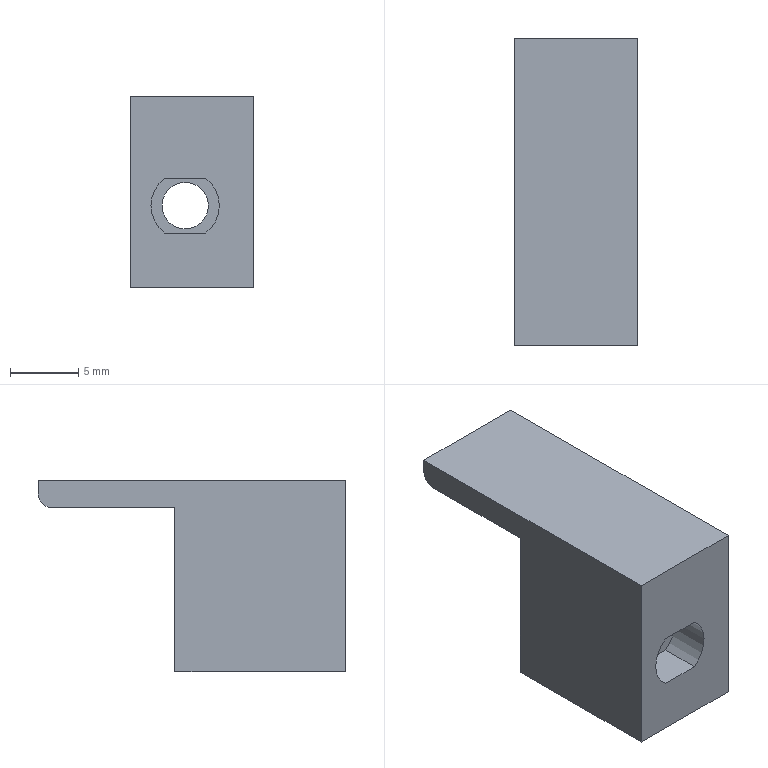Part | SolidWorks | features 3DProfileFeature 1, Cut 1, Extrusion 1, Fillet 1, HoleWzd 1, ICE 1 | 1 solid | 19 faces | box 9 x 22.5 x 14 mm | volume 1549 mm3 | plane 12 | cylinder 7 | commonest cylinder face diameters 3.4 x2 5 x2 6 x2 2 x1
STEP:
#1=CARTESIAN_POINT('',(-0.5,9.1,-4.));
#2=VERTEX_POINT('',#1);
#3=CARTESIAN_POINT('',(-0.5,9.1,2.));
#4=VERTEX_POINT('',#3);
#5=CARTESIAN_POINT('',(-0.5,9.1,-1.));
#6=DIRECTION('',(0.,1.,0.));
#7=DIRECTION('',(0.,0.,1.));
#8=AXIS2_PLACEMENT_3D('',#5,#6,#7);
#9=CIRCLE('',#8,3.);
#10=EDGE_CURVE('',#2,#4,#9,.T.);
#11=ORIENTED_EDGE('',*,*,#10,.F.);
#12=CARTESIAN_POINT('',(-0.5,12.5,-4.));
#13=VERTEX_POINT('',#12);
#14=CARTESIAN_POINT('',(-0.5,12.5,-4.));
#15=DIRECTION('',(0.,1.,0.));
#16=VECTOR('',#15,1000.);
#17=LINE('',#14,#16);
#18=EDGE_CURVE('',#2,#13,#17,.T.);
#19=ORIENTED_EDGE('',*,*,#18,.T.);
#20=CARTESIAN_POINT('',(-0.5,12.5,2.));
#21=VERTEX_POINT('',#20);
#22=CARTESIAN_POINT('',(-0.5,12.5,-1.));
#23=DIRECTION('',(0.,1.,0.));
#24=DIRECTION('',(0.,0.,1.));
#25=AXIS2_PLACEMENT_3D('',#22,#23,#24);
#26=CIRCLE('',#25,3.);
#27=EDGE_CURVE('',#13,#21,#26,.T.);
#28=ORIENTED_EDGE('',*,*,#27,.T.);
#29=CARTESIAN_POINT('',(-0.5,12.5,2.));
#30=DIRECTION('',(0.,1.,0.));
#31=VECTOR('',#30,1000.);
#32=LINE('',#29,#31);
#33=EDGE_CURVE('',#4,#21,#32,.T.);
#34=ORIENTED_EDGE('',*,*,#33,.F.);
#35=EDGE_LOOP('',(#11,#19,#28,#34));
#36=FACE_OUTER_BOUND('',#35,.T.);
#37=CARTESIAN_POINT('',(-0.5,12.5,-1.));
#38=DIRECTION('',(0.,1.,0.));
#39=DIRECTION('',(0.,0.,1.));
#40=AXIS2_PLACEMENT_3D('',#37,#38,#39);
#41=CYLINDRICAL_SURFACE('',#40,3.);
#42=ADVANCED_FACE('',(#36),#41,.F.);
#43=CARTESIAN_POINT('',(-0.5,3.,0.7));
#44=VERTEX_POINT('',#43);
#45=CARTESIAN_POINT('',(-0.5,3.,-2.7));
#46=VERTEX_POINT('',#45);
#47=CARTESIAN_POINT('',(-0.5,3.,-1.));
#48=DIRECTION('',(0.,-1.,0.));
#49=DIRECTION('',(0.,0.,-1.));
#50=AXIS2_PLACEMENT_3D('',#47,#48,#49);
#51=CIRCLE('',#50,1.7);
#52=EDGE_CURVE('',#44,#46,#51,.T.);
#53=ORIENTED_EDGE('',*,*,#52,.T.);
#54=CARTESIAN_POINT('',(-0.5,9.1,-2.7));
#55=VERTEX_POINT('',#54);
#56=CARTESIAN_POINT('',(-0.5,12.5,-2.7));
#57=DIRECTION('',(0.,1.,0.));
#58=VECTOR('',#57,1000.);
#59=LINE('',#56,#58);
#60=EDGE_CURVE('',#46,#55,#59,.T.);
#61=ORIENTED_EDGE('',*,*,#60,.T.);
#62=CARTESIAN_POINT('',(-0.5,9.1,0.7));
#63=VERTEX_POINT('',#62);
#64=CARTESIAN_POINT('',(-0.5,9.1,-1.));
#65=DIRECTION('',(0.,1.,0.));
#66=DIRECTION('',(0.,0.,1.));
#67=AXIS2_PLACEMENT_3D('',#64,#65,#66);
#68=CIRCLE('',#67,1.7);
#69=EDGE_CURVE('',#55,#63,#68,.T.);
#70=ORIENTED_EDGE('',*,*,#69,.T.);
#71=CARTESIAN_POINT('',(-0.5,12.5,0.7));
#72=DIRECTION('',(0.,1.,0.));
#73=VECTOR('',#72,1000.);
#74=LINE('',#71,#73);
#75=EDGE_CURVE('',#44,#63,#74,.T.);
#76=ORIENTED_EDGE('',*,*,#75,.F.);
#77=EDGE_LOOP('',(#53,#61,#70,#76));
#78=FACE_OUTER_BOUND('',#77,.T.);
#79=CARTESIAN_POINT('',(-0.5,12.5,-1.));
#80=DIRECTION('',(0.,1.,0.));
#81=DIRECTION('',(0.,0.,1.));
#82=AXIS2_PLACEMENT_3D('',#79,#80,#81);
#83=CYLINDRICAL_SURFACE('',#82,1.7);
#84=ADVANCED_FACE('',(#78),#83,.F.);
#85=CARTESIAN_POINT('',(-0.5,12.5,-1.));
#86=DIRECTION('',(0.,1.,0.));
#87=DIRECTION('',(0.,0.,1.));
#88=AXIS2_PLACEMENT_3D('',#85,#86,#87);
#89=CIRCLE('',#88,3.);
#90=EDGE_CURVE('',#21,#13,#89,.T.);
#91=ORIENTED_EDGE('',*,*,#90,.F.);
#92=ORIENTED_EDGE('',*,*,#27,.F.);
#93=EDGE_LOOP('',(#91,#92));
#94=FACE_BOUND('',#93,.T.);
#95=CARTESIAN_POINT('',(-4.5,12.5,-7.));
#96=VERTEX_POINT('',#95);
#97=CARTESIAN_POINT('',(-4.5,12.5,5.));
#98=VERTEX_POINT('',#97);
#99=CARTESIAN_POINT('',(-4.5,12.5,-7.));
#100=DIRECTION('',(0.,0.,1.));
#101=VECTOR('',#100,1000.);
#102=LINE('',#99,#101);
#103=EDGE_CURVE('',#96,#98,#102,.T.);
#104=ORIENTED_EDGE('',*,*,#103,.T.);
#105=CARTESIAN_POINT('',(4.5,12.5,5.));
#106=VERTEX_POINT('',#105);
#107=CARTESIAN_POINT('',(-4.5,12.5,5.));
#108=DIRECTION('',(1.,0.,0.));
#109=VECTOR('',#108,1000.);
#110=LINE('',#107,#109);
#111=EDGE_CURVE('',#98,#106,#110,.T.);
#112=ORIENTED_EDGE('',*,*,#111,.T.);
#113=CARTESIAN_POINT('',(4.5,12.5,-7.));
#114=VERTEX_POINT('',#113);
#115=CARTESIAN_POINT('',(4.5,12.5,-7.));
#116=DIRECTION('',(0.,0.,-1.));
#117=VECTOR('',#116,1000.);
#118=LINE('',#115,#117);
#119=EDGE_CURVE('',#106,#114,#118,.T.);
#120=ORIENTED_EDGE('',*,*,#119,.T.);
#121=CARTESIAN_POINT('',(-4.5,12.5,-7.));
#122=DIRECTION('',(-1.,0.,0.));
#123=VECTOR('',#122,1000.);
#124=LINE('',#121,#123);
#125=EDGE_CURVE('',#114,#96,#124,.T.);
#126=ORIENTED_EDGE('',*,*,#125,.T.);
#127=EDGE_LOOP('',(#104,#112,#120,#126));
#128=FACE_OUTER_BOUND('',#127,.T.);
#129=CARTESIAN_POINT('',(0.,12.5,0.));
#130=DIRECTION('',(0.,1.,0.));
#131=DIRECTION('',(0.,0.,1.));
#132=AXIS2_PLACEMENT_3D('',#129,#130,#131);
#133=PLANE('',#132);
#134=ADVANCED_FACE('',(#94,#128),#133,.T.);
#135=CARTESIAN_POINT('',(4.5,21.5,5.));
#136=VERTEX_POINT('',#135);
#137=CARTESIAN_POINT('',(4.5,12.5,5.));
#138=DIRECTION('',(0.,1.,0.));
#139=VECTOR('',#138,1000.);
#140=LINE('',#137,#139);
#141=EDGE_CURVE('',#106,#136,#140,.T.);
#142=ORIENTED_EDGE('',*,*,#141,.T.);
#143=CARTESIAN_POINT('',(4.5,22.5,6.));
#144=VERTEX_POINT('',#143);
#145=CARTESIAN_POINT('',(4.5,21.5,6.));
#146=DIRECTION('',(1.,0.,0.));
#147=DIRECTION('',(0.,0.,1.));
#148=AXIS2_PLACEMENT_3D('',#145,#146,#147);
#149=CIRCLE('',#148,1.);
#150=EDGE_CURVE('',#136,#144,#149,.T.);
#151=ORIENTED_EDGE('',*,*,#150,.T.);
#152=CARTESIAN_POINT('',(4.5,22.5,7.));
#153=VERTEX_POINT('',#152);
#154=CARTESIAN_POINT('',(4.5,22.5,5.));
#155=DIRECTION('',(0.,0.,1.));
#156=VECTOR('',#155,1000.);
#157=LINE('',#154,#156);
#158=EDGE_CURVE('',#144,#153,#157,.T.);
#159=ORIENTED_EDGE('',*,*,#158,.T.);
#160=CARTESIAN_POINT('',(4.5,0.,7.));
#161=VERTEX_POINT('',#160);
#162=CARTESIAN_POINT('',(4.5,12.5,7.));
#163=DIRECTION('',(0.,-1.,0.));
#164=VECTOR('',#163,1000.);
#165=LINE('',#162,#164);
#166=EDGE_CURVE('',#153,#161,#165,.T.);
#167=ORIENTED_EDGE('',*,*,#166,.T.);
#168=CARTESIAN_POINT('',(4.5,0.,-7.));
#169=VERTEX_POINT('',#168);
#170=CARTESIAN_POINT('',(4.5,0.,-7.));
#171=DIRECTION('',(0.,0.,-1.));
#172=VECTOR('',#171,1000.);
#173=LINE('',#170,#172);
#174=EDGE_CURVE('',#161,#169,#173,.T.);
#175=ORIENTED_EDGE('',*,*,#174,.T.);
#176=CARTESIAN_POINT('',(4.5,12.5,-7.));
#177=DIRECTION('',(0.,-1.,0.));
#178=VECTOR('',#177,1000.);
#179=LINE('',#176,#178);
#180=EDGE_CURVE('',#114,#169,#179,.T.);
#181=ORIENTED_EDGE('',*,*,#180,.F.);
#182=ORIENTED_EDGE('',*,*,#119,.F.);
#183=EDGE_LOOP('',(#142,#151,#159,#167,#175,#181,#182));
#184=FACE_OUTER_BOUND('',#183,.T.);
#185=CARTESIAN_POINT('',(4.5,12.5,-7.));
#186=DIRECTION('',(-1.,0.,0.));
#187=DIRECTION('',(0.,0.,1.));
#188=AXIS2_PLACEMENT_3D('',#185,#186,#187);
#189=PLANE('',#188);
#190=ADVANCED_FACE('',(#184),#189,.F.);
#191=CARTESIAN_POINT('',(-4.5,0.,-7.));
#192=VERTEX_POINT('',#191);
#193=CARTESIAN_POINT('',(-4.5,0.,-7.));
#194=DIRECTION('',(-1.,0.,0.));
#195=VECTOR('',#194,1000.);
#196=LINE('',#193,#195);
#197=EDGE_CURVE('',#169,#192,#196,.T.);
#198=ORIENTED_EDGE('',*,*,#197,.T.);
#199=CARTESIAN_POINT('',(-4.5,12.5,-7.));
#200=DIRECTION('',(0.,-1.,0.));
#201=VECTOR('',#200,1000.);
#202=LINE('',#199,#201);
#203=EDGE_CURVE('',#96,#192,#202,.T.);
#204=ORIENTED_EDGE('',*,*,#203,.F.);
#205=ORIENTED_EDGE('',*,*,#125,.F.);
#206=ORIENTED_EDGE('',*,*,#180,.T.);
#207=EDGE_LOOP('',(#198,#204,#205,#206));
#208=FACE_OUTER_BOUND('',#207,.T.);
#209=CARTESIAN_POINT('',(-4.5,12.5,-7.));
#210=DIRECTION('',(0.,0.,1.));
#211=DIRECTION('',(1.,0.,0.));
#212=AXIS2_PLACEMENT_3D('',#209,#210,#211);
#213=PLANE('',#212);
#214=ADVANCED_FACE('',(#208),#213,.F.);
#215=CARTESIAN_POINT('',(-4.5,22.5,6.));
#216=VERTEX_POINT('',#215);
#217=CARTESIAN_POINT('',(-4.5,22.5,7.));
#218=VERTEX_POINT('',#217);
#219=CARTESIAN_POINT('',(-4.5,22.5,5.));
#220=DIRECTION('',(0.,0.,1.));
#221=VECTOR('',#220,1000.);
#222=LINE('',#219,#221);
#223=EDGE_CURVE('',#216,#218,#222,.T.);
#224=ORIENTED_EDGE('',*,*,#223,.F.);
#225=CARTESIAN_POINT('',(-4.5,21.5,5.));
#226=VERTEX_POINT('',#225);
#227=CARTESIAN_POINT('',(-4.5,21.5,6.));
#228=DIRECTION('',(-1.,0.,0.));
#229=DIRECTION('',(0.,0.,-1.));
#230=AXIS2_PLACEMENT_3D('',#227,#228,#229);
#231=CIRCLE('',#230,1.);
#232=EDGE_CURVE('',#216,#226,#231,.T.);
#233=ORIENTED_EDGE('',*,*,#232,.T.);
#234=CARTESIAN_POINT('',(-4.5,12.5,5.));
#235=DIRECTION('',(0.,-1.,0.));
#236=VECTOR('',#235,1000.);
#237=LINE('',#234,#236);
#238=EDGE_CURVE('',#226,#98,#237,.T.);
#239=ORIENTED_EDGE('',*,*,#238,.T.);
#240=ORIENTED_EDGE('',*,*,#103,.F.);
#241=ORIENTED_EDGE('',*,*,#203,.T.);
#242=CARTESIAN_POINT('',(-4.5,0.,7.));
#243=VERTEX_POINT('',#242);
#244=CARTESIAN_POINT('',(-4.5,0.,-7.));
#245=DIRECTION('',(0.,0.,1.));
#246=VECTOR('',#245,1000.);
#247=LINE('',#244,#246);
#248=EDGE_CURVE('',#192,#243,#247,.T.);
#249=ORIENTED_EDGE('',*,*,#248,.T.);
#250=CARTESIAN_POINT('',(-4.5,12.5,7.));
#251=DIRECTION('',(0.,-1.,0.));
#252=VECTOR('',#251,1000.);
#253=LINE('',#250,#252);
#254=EDGE_CURVE('',#218,#243,#253,.T.);
#255=ORIENTED_EDGE('',*,*,#254,.F.);
#256=EDGE_LOOP('',(#224,#233,#239,#240,#241,#249,#255));
#257=FACE_OUTER_BOUND('',#256,.T.);
#258=CARTESIAN_POINT('',(-4.5,12.5,-7.));
#259=DIRECTION('',(1.,0.,0.));
#260=DIRECTION('',(0.,0.,-1.));
#261=AXIS2_PLACEMENT_3D('',#258,#259,#260);
#262=PLANE('',#261);
#263=ADVANCED_FACE('',(#257),#262,.F.);
#264=CARTESIAN_POINT('',(-4.5,0.,7.));
#265=DIRECTION('',(1.,0.,0.));
#266=VECTOR('',#265,1000.);
#267=LINE('',#264,#266);
#268=EDGE_CURVE('',#243,#161,#267,.T.);
#269=ORIENTED_EDGE('',*,*,#268,.T.);
#270=ORIENTED_EDGE('',*,*,#166,.F.);
#271=CARTESIAN_POINT('',(-4.5,22.5,7.));
#272=DIRECTION('',(-1.,0.,0.));
#273=VECTOR('',#272,1000.);
#274=LINE('',#271,#273);
#275=EDGE_CURVE('',#153,#218,#274,.T.);
#276=ORIENTED_EDGE('',*,*,#275,.T.);
#277=ORIENTED_EDGE('',*,*,#254,.T.);
#278=EDGE_LOOP('',(#269,#270,#276,#277));
#279=FACE_OUTER_BOUND('',#278,.T.);
#280=CARTESIAN_POINT('',(-4.5,12.5,7.));
#281=DIRECTION('',(0.,0.,-1.));
#282=DIRECTION('',(-1.,0.,0.));
#283=AXIS2_PLACEMENT_3D('',#280,#281,#282);
#284=PLANE('',#283);
#285=ADVANCED_FACE('',(#279),#284,.F.);
#286=CARTESIAN_POINT('',(-2.,0.,-3.));
#287=VERTEX_POINT('',#286);
#288=CARTESIAN_POINT('',(1.,0.,-3.));
#289=VERTEX_POINT('',#288);
#290=CARTESIAN_POINT('',(-2.,0.,-3.));
#291=DIRECTION('',(1.,0.,0.));
#292=VECTOR('',#291,1000.);
#293=LINE('',#290,#292);
#294=EDGE_CURVE('',#287,#289,#293,.T.);
#295=ORIENTED_EDGE('',*,*,#294,.F.);
#296=CARTESIAN_POINT('',(-2.,0.,1.));
#297=VERTEX_POINT('',#296);
#298=CARTESIAN_POINT('',(-0.5,0.,-1.));
#299=DIRECTION('',(0.,-1.,0.));
#300=DIRECTION('',(0.,0.,-1.));
#301=AXIS2_PLACEMENT_3D('',#298,#299,#300);
#302=CIRCLE('',#301,2.5);
#303=EDGE_CURVE('',#297,#287,#302,.T.);
#304=ORIENTED_EDGE('',*,*,#303,.F.);
#305=CARTESIAN_POINT('',(1.,0.,1.));
#306=VERTEX_POINT('',#305);
#307=CARTESIAN_POINT('',(1.,0.,1.));
#308=DIRECTION('',(-1.,0.,0.));
#309=VECTOR('',#308,1000.);
#310=LINE('',#307,#309);
#311=EDGE_CURVE('',#306,#297,#310,.T.);
#312=ORIENTED_EDGE('',*,*,#311,.F.);
#313=CARTESIAN_POINT('',(-0.5,0.,-1.));
#314=DIRECTION('',(0.,-1.,0.));
#315=DIRECTION('',(0.,0.,-1.));
#316=AXIS2_PLACEMENT_3D('',#313,#314,#315);
#317=CIRCLE('',#316,2.5);
#318=EDGE_CURVE('',#289,#306,#317,.T.);
#319=ORIENTED_EDGE('',*,*,#318,.F.);
#320=EDGE_LOOP('',(#295,#304,#312,#319));
#321=FACE_BOUND('',#320,.T.);
#322=ORIENTED_EDGE('',*,*,#174,.F.);
#323=ORIENTED_EDGE('',*,*,#268,.F.);
#324=ORIENTED_EDGE('',*,*,#248,.F.);
#325=ORIENTED_EDGE('',*,*,#197,.F.);
#326=EDGE_LOOP('',(#322,#323,#324,#325));
#327=FACE_OUTER_BOUND('',#326,.T.);
#328=CARTESIAN_POINT('',(0.,0.,0.));
#329=DIRECTION('',(0.,1.,0.));
#330=DIRECTION('',(0.,0.,1.));
#331=AXIS2_PLACEMENT_3D('',#328,#329,#330);
#332=PLANE('',#331);
#333=ADVANCED_FACE('',(#321,#327),#332,.F.);
#334=ORIENTED_EDGE('',*,*,#303,.T.);
#335=CARTESIAN_POINT('',(-2.,3.,-3.));
#336=VERTEX_POINT('',#335);
#337=CARTESIAN_POINT('',(-2.,3.,-3.));
#338=DIRECTION('',(0.,-1.,0.));
#339=VECTOR('',#338,1000.);
#340=LINE('',#337,#339);
#341=EDGE_CURVE('',#336,#287,#340,.T.);
#342=ORIENTED_EDGE('',*,*,#341,.F.);
#343=CARTESIAN_POINT('',(-2.,3.,1.));
#344=VERTEX_POINT('',#343);
#345=CARTESIAN_POINT('',(-0.5,3.,-1.));
#346=DIRECTION('',(0.,-1.,0.));
#347=DIRECTION('',(0.,0.,-1.));
#348=AXIS2_PLACEMENT_3D('',#345,#346,#347);
#349=CIRCLE('',#348,2.5);
#350=EDGE_CURVE('',#344,#336,#349,.T.);
#351=ORIENTED_EDGE('',*,*,#350,.F.);
#352=CARTESIAN_POINT('',(-2.,3.,1.));
#353=DIRECTION('',(0.,-1.,0.));
#354=VECTOR('',#353,1000.);
#355=LINE('',#352,#354);
#356=EDGE_CURVE('',#344,#297,#355,.T.);
#357=ORIENTED_EDGE('',*,*,#356,.T.);
#358=EDGE_LOOP('',(#334,#342,#351,#357));
#359=FACE_OUTER_BOUND('',#358,.T.);
#360=CARTESIAN_POINT('',(-0.5,3.,-1.));
#361=DIRECTION('',(0.,-1.,0.));
#362=DIRECTION('',(0.,0.,-1.));
#363=AXIS2_PLACEMENT_3D('',#360,#361,#362);
#364=CYLINDRICAL_SURFACE('',#363,2.5);
#365=ADVANCED_FACE('',(#359),#364,.F.);
#366=ORIENTED_EDGE('',*,*,#311,.T.);
#367=ORIENTED_EDGE('',*,*,#356,.F.);
#368=CARTESIAN_POINT('',(1.,3.,1.));
#369=VERTEX_POINT('',#368);
#370=CARTESIAN_POINT('',(1.,3.,1.));
#371=DIRECTION('',(-1.,0.,0.));
#372=VECTOR('',#371,1000.);
#373=LINE('',#370,#372);
#374=EDGE_CURVE('',#369,#344,#373,.T.);
#375=ORIENTED_EDGE('',*,*,#374,.F.);
#376=CARTESIAN_POINT('',(1.,3.,1.));
#377=DIRECTION('',(0.,-1.,0.));
#378=VECTOR('',#377,1000.);
#379=LINE('',#376,#378);
#380=EDGE_CURVE('',#369,#306,#379,.T.);
#381=ORIENTED_EDGE('',*,*,#380,.T.);
#382=EDGE_LOOP('',(#366,#367,#375,#381));
#383=FACE_OUTER_BOUND('',#382,.T.);
#384=CARTESIAN_POINT('',(1.,3.,1.));
#385=DIRECTION('',(0.,0.,1.));
#386=DIRECTION('',(1.,0.,0.));
#387=AXIS2_PLACEMENT_3D('',#384,#385,#386);
#388=PLANE('',#387);
#389=ADVANCED_FACE('',(#383),#388,.F.);
#390=ORIENTED_EDGE('',*,*,#318,.T.);
#391=ORIENTED_EDGE('',*,*,#380,.F.);
#392=CARTESIAN_POINT('',(1.,3.,-3.));
#393=VERTEX_POINT('',#392);
#394=CARTESIAN_POINT('',(-0.5,3.,-1.));
#395=DIRECTION('',(0.,-1.,0.));
#396=DIRECTION('',(0.,0.,-1.));
#397=AXIS2_PLACEMENT_3D('',#394,#395,#396);
#398=CIRCLE('',#397,2.5);
#399=EDGE_CURVE('',#393,#369,#398,.T.);
#400=ORIENTED_EDGE('',*,*,#399,.F.);
#401=CARTESIAN_POINT('',(1.,3.,-3.));
#402=DIRECTION('',(0.,-1.,0.));
#403=VECTOR('',#402,1000.);
#404=LINE('',#401,#403);
#405=EDGE_CURVE('',#393,#289,#404,.T.);
#406=ORIENTED_EDGE('',*,*,#405,.T.);
#407=EDGE_LOOP('',(#390,#391,#400,#406));
#408=FACE_OUTER_BOUND('',#407,.T.);
#409=CARTESIAN_POINT('',(-0.5,3.,-1.));
#410=DIRECTION('',(0.,-1.,0.));
#411=DIRECTION('',(0.,0.,-1.));
#412=AXIS2_PLACEMENT_3D('',#409,#410,#411);
#413=CYLINDRICAL_SURFACE('',#412,2.5);
#414=ADVANCED_FACE('',(#408),#413,.F.);
#415=ORIENTED_EDGE('',*,*,#294,.T.);
#416=ORIENTED_EDGE('',*,*,#405,.F.);
#417=CARTESIAN_POINT('',(-2.,3.,-3.));
#418=DIRECTION('',(1.,0.,0.));
#419=VECTOR('',#418,1000.);
#420=LINE('',#417,#419);
#421=EDGE_CURVE('',#336,#393,#420,.T.);
#422=ORIENTED_EDGE('',*,*,#421,.F.);
#423=ORIENTED_EDGE('',*,*,#341,.T.);
#424=EDGE_LOOP('',(#415,#416,#422,#423));
#425=FACE_OUTER_BOUND('',#424,.T.);
#426=CARTESIAN_POINT('',(-2.,3.,-3.));
#427=DIRECTION('',(0.,0.,-1.));
#428=DIRECTION('',(-1.,0.,0.));
#429=AXIS2_PLACEMENT_3D('',#426,#427,#428);
#430=PLANE('',#429);
#431=ADVANCED_FACE('',(#425),#430,.F.);
#432=ORIENTED_EDGE('',*,*,#52,.F.);
#433=CARTESIAN_POINT('',(-0.5,3.,-1.));
#434=DIRECTION('',(0.,-1.,0.));
#435=DIRECTION('',(0.,0.,-1.));
#436=AXIS2_PLACEMENT_3D('',#433,#434,#435);
#437=CIRCLE('',#436,1.7);
#438=EDGE_CURVE('',#46,#44,#437,.T.);
#439=ORIENTED_EDGE('',*,*,#438,.F.);
#440=EDGE_LOOP('',(#432,#439));
#441=FACE_BOUND('',#440,.T.);
#442=ORIENTED_EDGE('',*,*,#350,.T.);
#443=ORIENTED_EDGE('',*,*,#421,.T.);
#444=ORIENTED_EDGE('',*,*,#399,.T.);
#445=ORIENTED_EDGE('',*,*,#374,.T.);
#446=EDGE_LOOP('',(#442,#443,#444,#445));
#447=FACE_OUTER_BOUND('',#446,.T.);
#448=CARTESIAN_POINT('',(-0.5,3.,-1.));
#449=DIRECTION('',(0.,-1.,0.));
#450=DIRECTION('',(0.,0.,-1.));
#451=AXIS2_PLACEMENT_3D('',#448,#449,#450);
#452=PLANE('',#451);
#453=ADVANCED_FACE('',(#441,#447),#452,.T.);
#454=ORIENTED_EDGE('',*,*,#158,.F.);
#455=CARTESIAN_POINT('',(-4.5,22.5,6.));
#456=DIRECTION('',(-1.,0.,0.));
#457=VECTOR('',#456,1000.);
#458=LINE('',#455,#457);
#459=EDGE_CURVE('',#144,#216,#458,.T.);
#460=ORIENTED_EDGE('',*,*,#459,.T.);
#461=ORIENTED_EDGE('',*,*,#223,.T.);
#462=ORIENTED_EDGE('',*,*,#275,.F.);
#463=EDGE_LOOP('',(#454,#460,#461,#462));
#464=FACE_OUTER_BOUND('',#463,.T.);
#465=CARTESIAN_POINT('',(-4.5,22.5,5.));
#466=DIRECTION('',(0.,1.,0.));
#467=DIRECTION('',(0.,0.,1.));
#468=AXIS2_PLACEMENT_3D('',#465,#466,#467);
#469=PLANE('',#468);
#470=ADVANCED_FACE('',(#464),#469,.T.);
#471=ORIENTED_EDGE('',*,*,#238,.F.);
#472=CARTESIAN_POINT('',(0.,21.5,5.));
#473=DIRECTION('',(1.,0.,0.));
#474=VECTOR('',#473,1000.);
#475=LINE('',#472,#474);
#476=EDGE_CURVE('',#226,#136,#475,.T.);
#477=ORIENTED_EDGE('',*,*,#476,.T.);
#478=ORIENTED_EDGE('',*,*,#141,.F.);
#479=ORIENTED_EDGE('',*,*,#111,.F.);
#480=EDGE_LOOP('',(#471,#477,#478,#479));
#481=FACE_OUTER_BOUND('',#480,.T.);
#482=CARTESIAN_POINT('',(0.,0.,5.));
#483=DIRECTION('',(0.,0.,-1.));
#484=DIRECTION('',(-1.,0.,0.));
#485=AXIS2_PLACEMENT_3D('',#482,#483,#484);
#486=PLANE('',#485);
#487=ADVANCED_FACE('',(#481),#486,.T.);
#488=ORIENTED_EDGE('',*,*,#150,.F.);
#489=ORIENTED_EDGE('',*,*,#476,.F.);
#490=ORIENTED_EDGE('',*,*,#232,.F.);
#491=ORIENTED_EDGE('',*,*,#459,.F.);
#492=EDGE_LOOP('',(#488,#489,#490,#491));
#493=FACE_OUTER_BOUND('',#492,.T.);
#494=CARTESIAN_POINT('',(-4.5,21.5,6.));
#495=DIRECTION('',(-1.,0.,0.));
#496=DIRECTION('',(0.,0.,1.));
#497=AXIS2_PLACEMENT_3D('',#494,#495,#496);
#498=CYLINDRICAL_SURFACE('',#497,1.);
#499=ADVANCED_FACE('',(#493),#498,.T.);
#500=ORIENTED_EDGE('',*,*,#60,.F.);
#501=ORIENTED_EDGE('',*,*,#438,.T.);
#502=ORIENTED_EDGE('',*,*,#75,.T.);
#503=CARTESIAN_POINT('',(-0.5,9.1,-1.));
#504=DIRECTION('',(0.,1.,0.));
#505=DIRECTION('',(0.,0.,1.));
#506=AXIS2_PLACEMENT_3D('',#503,#504,#505);
#507=CIRCLE('',#506,1.7);
#508=EDGE_CURVE('',#63,#55,#507,.T.);
#509=ORIENTED_EDGE('',*,*,#508,.T.);
#510=EDGE_LOOP('',(#500,#501,#502,#509));
#511=FACE_OUTER_BOUND('',#510,.T.);
#512=CARTESIAN_POINT('',(-0.5,12.5,-1.));
#513=DIRECTION('',(0.,1.,0.));
#514=DIRECTION('',(0.,0.,1.));
#515=AXIS2_PLACEMENT_3D('',#512,#513,#514);
#516=CYLINDRICAL_SURFACE('',#515,1.7);
#517=ADVANCED_FACE('',(#511),#516,.F.);
#518=ORIENTED_EDGE('',*,*,#508,.F.);
#519=ORIENTED_EDGE('',*,*,#69,.F.);
#520=EDGE_LOOP('',(#518,#519));
#521=FACE_BOUND('',#520,.T.);
#522=CARTESIAN_POINT('',(-0.5,9.1,-1.));
#523=DIRECTION('',(0.,1.,0.));
#524=DIRECTION('',(0.,0.,1.));
#525=AXIS2_PLACEMENT_3D('',#522,#523,#524);
#526=CIRCLE('',#525,3.);
#527=EDGE_CURVE('',#4,#2,#526,.T.);
#528=ORIENTED_EDGE('',*,*,#527,.T.);
#529=ORIENTED_EDGE('',*,*,#10,.T.);
#530=EDGE_LOOP('',(#528,#529));
#531=FACE_OUTER_BOUND('',#530,.T.);
#532=CARTESIAN_POINT('',(1.2,9.1,-1.));
#533=DIRECTION('',(0.,-1.,0.));
#534=DIRECTION('',(0.,0.,-1.));
#535=AXIS2_PLACEMENT_3D('',#532,#533,#534);
#536=PLANE('',#535);
#537=ADVANCED_FACE('',(#521,#531),#536,.F.);
#538=ORIENTED_EDGE('',*,*,#18,.F.);
#539=ORIENTED_EDGE('',*,*,#527,.F.);
#540=ORIENTED_EDGE('',*,*,#33,.T.);
#541=ORIENTED_EDGE('',*,*,#90,.T.);
#542=EDGE_LOOP('',(#538,#539,#540,#541));
#543=FACE_OUTER_BOUND('',#542,.T.);
#544=CARTESIAN_POINT('',(-0.5,12.5,-1.));
#545=DIRECTION('',(0.,1.,0.));
#546=DIRECTION('',(0.,0.,1.));
#547=AXIS2_PLACEMENT_3D('',#544,#545,#546);
#548=CYLINDRICAL_SURFACE('',#547,3.);
#549=ADVANCED_FACE('',(#543),#548,.F.);
#550=CLOSED_SHELL('',(#42,#84,#134,#190,#214,#263,#285,#333,#365,#389,#414,#431,#453,#470,#487,#499,#517,#537,#549));
#551=MANIFOLD_SOLID_BREP('',#550);
#552=CARTESIAN_POINT('',(0.,0.,0.));
#553=DIRECTION('',(0.,0.,1.));
#554=DIRECTION('',(1.,0.,0.));
#555=AXIS2_PLACEMENT_3D('',#552,#553,#554);
#556=(LENGTH_UNIT()NAMED_UNIT(*)SI_UNIT(.MILLI.,.METRE.));
#557=UNCERTAINTY_MEASURE_WITH_UNIT(LENGTH_MEASURE(0.00001),#556,'','');
#558=(NAMED_UNIT(*)PLANE_ANGLE_UNIT()SI_UNIT($,.RADIAN.));
#559=(NAMED_UNIT(*)SI_UNIT($,.STERADIAN.)SOLID_ANGLE_UNIT());
#560=(GEOMETRIC_REPRESENTATION_CONTEXT(3)GLOBAL_UNCERTAINTY_ASSIGNED_CONTEXT((#557))GLOBAL_UNIT_ASSIGNED_CONTEXT((#556,#558,#559))REPRESENTATION_CONTEXT('',''));
#561=ADVANCED_BREP_SHAPE_REPRESENTATION('',(#551,#555),#560);